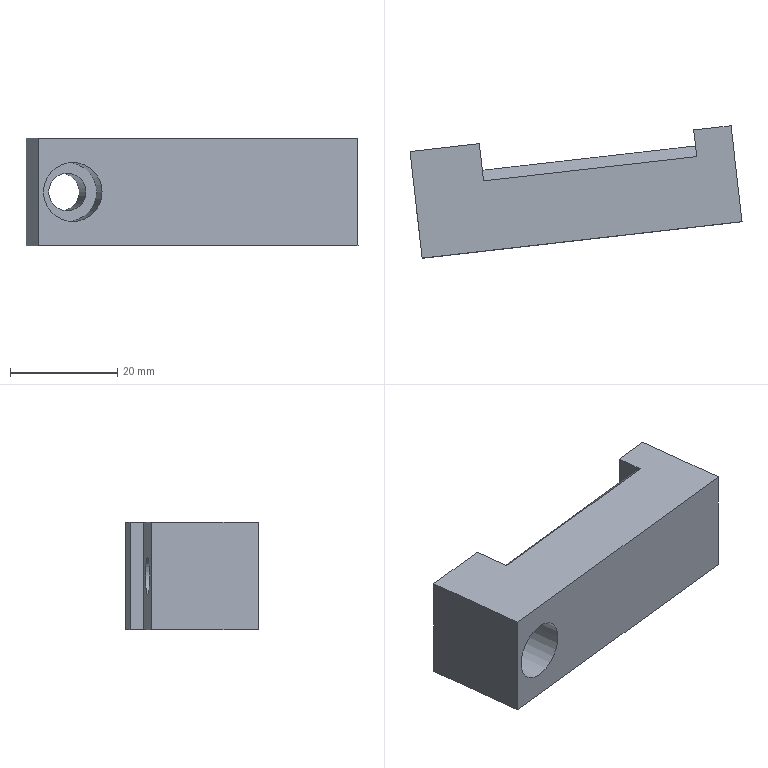Part | NX | features XQ 2 | 1 solid | 15 faces | box 61.878 x 24.676 x 20 mm | volume 18281 mm3 | plane 13 | cylinder 2 | commonest cylinder face diameters 7 x1 11 x1
STEP:
#1=CARTESIAN_POINT('',(3280.526,214.819,-94.126));
#2=VERTEX_POINT('',#1);
#3=CARTESIAN_POINT('',(3220.911,208.026,-94.126));
#4=VERTEX_POINT('',#3);
#5=CARTESIAN_POINT('',(3240.783,210.291,-94.126));
#6=DIRECTION('',(-0.9936,-0.1132,0.));
#7=VECTOR('',#6,1000.);
#8=LINE('',#5,#7);
#9=EDGE_CURVE('',#2,#4,#8,.T.);
#10=ORIENTED_EDGE('',*,*,#9,.F.);
#11=CARTESIAN_POINT('',(3280.526,214.819,-74.126));
#12=VERTEX_POINT('',#11);
#13=CARTESIAN_POINT('',(3280.526,214.819,-148.027));
#14=DIRECTION('',(0.,0.,-1.));
#15=VECTOR('',#14,1000.);
#16=LINE('',#13,#15);
#17=EDGE_CURVE('',#12,#2,#16,.T.);
#18=ORIENTED_EDGE('',*,*,#17,.F.);
#19=CARTESIAN_POINT('',(3220.911,208.026,-74.126));
#20=VERTEX_POINT('',#19);
#21=CARTESIAN_POINT('',(3240.783,210.291,-74.126));
#22=DIRECTION('',(0.9936,0.1132,0.));
#23=VECTOR('',#22,1000.);
#24=LINE('',#21,#23);
#25=EDGE_CURVE('',#20,#12,#24,.T.);
#26=ORIENTED_EDGE('',*,*,#25,.F.);
#27=CARTESIAN_POINT('',(3220.911,208.026,-94.126));
#28=DIRECTION('',(0.,0.,-1.));
#29=VECTOR('',#28,1000.);
#30=LINE('',#27,#29);
#31=EDGE_CURVE('',#20,#4,#30,.T.);
#32=ORIENTED_EDGE('',*,*,#31,.T.);
#33=EDGE_LOOP('',(#10,#18,#26,#32));
#34=FACE_BOUND('',#33,.T.);
#35=CARTESIAN_POINT('',(3232.834,209.385,-84.126));
#36=VERTEX_POINT('',#35);
#37=CARTESIAN_POINT('',(3227.369,208.762,-84.126));
#38=DIRECTION('',(0.1132,-0.9936,0.));
#39=DIRECTION('',(0.9936,0.1132,0.));
#40=AXIS2_PLACEMENT_3D('',#37,#38,#39);
#41=CIRCLE('',#40,5.5);
#42=EDGE_CURVE('',#36,#36,#41,.T.);
#43=ORIENTED_EDGE('',*,*,#42,.F.);
#44=EDGE_LOOP('',(#43));
#45=FACE_BOUND('',#44,.T.);
#46=CARTESIAN_POINT('',(3240.783,210.291,-94.126));
#47=DIRECTION('',(0.1132,-0.9936,0.));
#48=DIRECTION('',(0.9936,0.1132,0.));
#49=AXIS2_PLACEMENT_3D('',#46,#47,#48);
#50=PLANE('',#49);
#51=ADVANCED_FACE('',(#34,#45),#50,.T.);
#52=CARTESIAN_POINT('',(3231.564,229.37,-74.126));
#53=VERTEX_POINT('',#52);
#54=CARTESIAN_POINT('',(3218.647,227.898,-74.126));
#55=VERTEX_POINT('',#54);
#56=CARTESIAN_POINT('',(3236.531,229.936,-74.126));
#57=DIRECTION('',(-0.9936,-0.1132,0.));
#58=VECTOR('',#57,1000.);
#59=LINE('',#56,#58);
#60=EDGE_CURVE('',#53,#55,#59,.T.);
#61=ORIENTED_EDGE('',*,*,#60,.F.);
#62=CARTESIAN_POINT('',(3231.564,229.37,-94.126));
#63=VERTEX_POINT('',#62);
#64=CARTESIAN_POINT('',(3231.564,229.37,-94.126));
#65=DIRECTION('',(0.,0.,1.));
#66=VECTOR('',#65,1000.);
#67=LINE('',#64,#66);
#68=EDGE_CURVE('',#63,#53,#67,.T.);
#69=ORIENTED_EDGE('',*,*,#68,.F.);
#70=CARTESIAN_POINT('',(3218.647,227.898,-94.126));
#71=VERTEX_POINT('',#70);
#72=CARTESIAN_POINT('',(3236.531,229.936,-94.126));
#73=DIRECTION('',(0.9936,0.1132,0.));
#74=VECTOR('',#73,1000.);
#75=LINE('',#72,#74);
#76=EDGE_CURVE('',#71,#63,#75,.T.);
#77=ORIENTED_EDGE('',*,*,#76,.F.);
#78=CARTESIAN_POINT('',(3218.647,227.898,-94.126));
#79=DIRECTION('',(0.,0.,-1.));
#80=VECTOR('',#79,1000.);
#81=LINE('',#78,#80);
#82=EDGE_CURVE('',#55,#71,#81,.T.);
#83=ORIENTED_EDGE('',*,*,#82,.F.);
#84=EDGE_LOOP('',(#61,#69,#77,#83));
#85=FACE_BOUND('',#84,.T.);
#86=CARTESIAN_POINT('',(3221.628,228.237,-84.126));
#87=VERTEX_POINT('',#86);
#88=CARTESIAN_POINT('',(3225.105,228.634,-84.126));
#89=DIRECTION('',(-0.1132,0.9936,0.));
#90=DIRECTION('',(-0.9936,-0.1132,0.));
#91=AXIS2_PLACEMENT_3D('',#88,#89,#90);
#92=CIRCLE('',#91,3.5);
#93=EDGE_CURVE('',#87,#87,#92,.T.);
#94=ORIENTED_EDGE('',*,*,#93,.F.);
#95=EDGE_LOOP('',(#94));
#96=FACE_BOUND('',#95,.T.);
#97=CARTESIAN_POINT('',(3236.531,229.936,-94.126));
#98=DIRECTION('',(-0.1132,0.9936,0.));
#99=DIRECTION('',(-0.9936,-0.1132,0.));
#100=AXIS2_PLACEMENT_3D('',#97,#98,#99);
#101=PLANE('',#100);
#102=ADVANCED_FACE('',(#85,#96),#101,.T.);
#103=CARTESIAN_POINT('',(3272.099,226.943,-74.126));
#104=VERTEX_POINT('',#103);
#105=CARTESIAN_POINT('',(3232.356,222.415,-74.126));
#106=VERTEX_POINT('',#105);
#107=CARTESIAN_POINT('',(3239.311,223.207,-74.126));
#108=DIRECTION('',(-0.9936,-0.1132,0.));
#109=VECTOR('',#108,1000.);
#110=LINE('',#107,#109);
#111=EDGE_CURVE('',#104,#106,#110,.T.);
#112=ORIENTED_EDGE('',*,*,#111,.T.);
#113=CARTESIAN_POINT('',(3232.696,219.434,-74.126));
#114=DIRECTION('',(-0.1132,0.9936,0.));
#115=VECTOR('',#114,1000.);
#116=LINE('',#113,#115);
#117=EDGE_CURVE('',#106,#53,#116,.T.);
#118=ORIENTED_EDGE('',*,*,#117,.T.);
#119=ORIENTED_EDGE('',*,*,#60,.T.);
#120=CARTESIAN_POINT('',(3219.779,217.962,-74.126));
#121=DIRECTION('',(0.1132,-0.9936,0.));
#122=VECTOR('',#121,1000.);
#123=LINE('',#120,#122);
#124=EDGE_CURVE('',#55,#20,#123,.T.);
#125=ORIENTED_EDGE('',*,*,#124,.T.);
#126=ORIENTED_EDGE('',*,*,#25,.T.);
#127=CARTESIAN_POINT('',(3278.488,232.703,-74.126));
#128=VERTEX_POINT('',#127);
#129=CARTESIAN_POINT('',(3279.394,224.754,-74.126));
#130=DIRECTION('',(-0.1132,0.9936,0.));
#131=VECTOR('',#130,1000.);
#132=LINE('',#129,#131);
#133=EDGE_CURVE('',#12,#128,#132,.T.);
#134=ORIENTED_EDGE('',*,*,#133,.T.);
#135=CARTESIAN_POINT('',(3271.533,231.91,-74.126));
#136=VERTEX_POINT('',#135);
#137=CARTESIAN_POINT('',(3238.745,228.175,-74.126));
#138=DIRECTION('',(-0.9936,-0.1132,0.));
#139=VECTOR('',#138,1000.);
#140=LINE('',#137,#139);
#141=EDGE_CURVE('',#128,#136,#140,.T.);
#142=ORIENTED_EDGE('',*,*,#141,.T.);
#143=CARTESIAN_POINT('',(3272.439,223.962,-74.126));
#144=DIRECTION('',(0.1132,-0.9936,0.));
#145=VECTOR('',#144,1000.);
#146=LINE('',#143,#145);
#147=EDGE_CURVE('',#136,#104,#146,.T.);
#148=ORIENTED_EDGE('',*,*,#147,.T.);
#149=EDGE_LOOP('',(#112,#118,#119,#125,#126,#134,#142,#148));
#150=FACE_BOUND('',#149,.T.);
#151=CARTESIAN_POINT('',(3239.651,220.226,-74.126));
#152=DIRECTION('',(0.,0.,1.));
#153=DIRECTION('',(-0.9981,0.06105,0.));
#154=AXIS2_PLACEMENT_3D('',#151,#152,#153);
#155=PLANE('',#154);
#156=ADVANCED_FACE('',(#150),#155,.T.);
#157=CARTESIAN_POINT('',(3271.873,228.93,-76.126));
#158=VERTEX_POINT('',#157);
#159=CARTESIAN_POINT('',(3271.873,228.93,-92.126));
#160=VERTEX_POINT('',#159);
#161=CARTESIAN_POINT('',(3271.873,228.93,-84.126));
#162=DIRECTION('',(0.,0.,-1.));
#163=VECTOR('',#162,1000.);
#164=LINE('',#161,#163);
#165=EDGE_CURVE('',#158,#160,#164,.T.);
#166=ORIENTED_EDGE('',*,*,#165,.T.);
#167=CARTESIAN_POINT('',(3232.13,224.402,-92.126));
#168=VERTEX_POINT('',#167);
#169=CARTESIAN_POINT('',(3239.085,225.194,-92.126));
#170=DIRECTION('',(-0.9936,-0.1132,0.));
#171=VECTOR('',#170,1000.);
#172=LINE('',#169,#171);
#173=EDGE_CURVE('',#160,#168,#172,.T.);
#174=ORIENTED_EDGE('',*,*,#173,.T.);
#175=CARTESIAN_POINT('',(3232.13,224.402,-76.126));
#176=VERTEX_POINT('',#175);
#177=CARTESIAN_POINT('',(3232.13,224.402,-84.126));
#178=DIRECTION('',(0.,0.,-1.));
#179=VECTOR('',#178,1000.);
#180=LINE('',#177,#179);
#181=EDGE_CURVE('',#176,#168,#180,.T.);
#182=ORIENTED_EDGE('',*,*,#181,.F.);
#183=CARTESIAN_POINT('',(3239.085,225.194,-76.126));
#184=DIRECTION('',(0.9936,0.1132,0.));
#185=VECTOR('',#184,1000.);
#186=LINE('',#183,#185);
#187=EDGE_CURVE('',#176,#158,#186,.T.);
#188=ORIENTED_EDGE('',*,*,#187,.T.);
#189=EDGE_LOOP('',(#166,#174,#182,#188));
#190=FACE_BOUND('',#189,.T.);
#191=CARTESIAN_POINT('',(3239.085,225.194,-94.126));
#192=DIRECTION('',(-0.1132,0.9936,0.));
#193=DIRECTION('',(-0.9936,-0.1132,0.));
#194=AXIS2_PLACEMENT_3D('',#191,#192,#193);
#195=PLANE('',#194);
#196=ADVANCED_FACE('',(#190),#195,.T.);
#197=CARTESIAN_POINT('',(3232.356,222.415,-94.126));
#198=VERTEX_POINT('',#197);
#199=CARTESIAN_POINT('',(3272.099,226.943,-94.126));
#200=VERTEX_POINT('',#199);
#201=CARTESIAN_POINT('',(3239.311,223.207,-94.126));
#202=DIRECTION('',(0.9936,0.1132,0.));
#203=VECTOR('',#202,1000.);
#204=LINE('',#201,#203);
#205=EDGE_CURVE('',#198,#200,#204,.T.);
#206=ORIENTED_EDGE('',*,*,#205,.T.);
#207=CARTESIAN_POINT('',(3271.533,231.91,-94.126));
#208=VERTEX_POINT('',#207);
#209=CARTESIAN_POINT('',(3272.439,223.962,-94.126));
#210=DIRECTION('',(0.1132,-0.9936,0.));
#211=VECTOR('',#210,1000.);
#212=LINE('',#209,#211);
#213=EDGE_CURVE('',#208,#200,#212,.T.);
#214=ORIENTED_EDGE('',*,*,#213,.F.);
#215=CARTESIAN_POINT('',(3278.488,232.703,-94.126));
#216=VERTEX_POINT('',#215);
#217=CARTESIAN_POINT('',(3238.745,228.175,-94.126));
#218=DIRECTION('',(0.9936,0.1132,0.));
#219=VECTOR('',#218,1000.);
#220=LINE('',#217,#219);
#221=EDGE_CURVE('',#208,#216,#220,.T.);
#222=ORIENTED_EDGE('',*,*,#221,.T.);
#223=CARTESIAN_POINT('',(3279.394,224.754,-94.126));
#224=DIRECTION('',(0.1132,-0.9936,0.));
#225=VECTOR('',#224,1000.);
#226=LINE('',#223,#225);
#227=EDGE_CURVE('',#216,#2,#226,.T.);
#228=ORIENTED_EDGE('',*,*,#227,.T.);
#229=ORIENTED_EDGE('',*,*,#9,.T.);
#230=CARTESIAN_POINT('',(3219.779,217.962,-94.126));
#231=DIRECTION('',(-0.1132,0.9936,0.));
#232=VECTOR('',#231,1000.);
#233=LINE('',#230,#232);
#234=EDGE_CURVE('',#4,#71,#233,.T.);
#235=ORIENTED_EDGE('',*,*,#234,.T.);
#236=ORIENTED_EDGE('',*,*,#76,.T.);
#237=CARTESIAN_POINT('',(3232.696,219.434,-94.126));
#238=DIRECTION('',(0.1132,-0.9936,0.));
#239=VECTOR('',#238,1000.);
#240=LINE('',#237,#239);
#241=EDGE_CURVE('',#63,#198,#240,.T.);
#242=ORIENTED_EDGE('',*,*,#241,.T.);
#243=EDGE_LOOP('',(#206,#214,#222,#228,#229,#235,#236,#242));
#244=FACE_BOUND('',#243,.T.);
#245=CARTESIAN_POINT('',(3239.651,220.226,-94.126));
#246=DIRECTION('',(0.,0.,-1.));
#247=DIRECTION('',(0.9981,-0.06105,0.));
#248=AXIS2_PLACEMENT_3D('',#245,#246,#247);
#249=PLANE('',#248);
#250=ADVANCED_FACE('',(#244),#249,.T.);
#251=ORIENTED_EDGE('',*,*,#241,.F.);
#252=ORIENTED_EDGE('',*,*,#68,.T.);
#253=ORIENTED_EDGE('',*,*,#117,.F.);
#254=CARTESIAN_POINT('',(3232.356,222.415,-74.126));
#255=DIRECTION('',(-0.08005,0.7026,-0.7071));
#256=VECTOR('',#255,1000.);
#257=LINE('',#254,#256);
#258=EDGE_CURVE('',#106,#176,#257,.T.);
#259=ORIENTED_EDGE('',*,*,#258,.T.);
#260=ORIENTED_EDGE('',*,*,#181,.T.);
#261=CARTESIAN_POINT('',(3232.356,222.415,-94.126));
#262=DIRECTION('',(0.08005,-0.7026,-0.7071));
#263=VECTOR('',#262,1000.);
#264=LINE('',#261,#263);
#265=EDGE_CURVE('',#168,#198,#264,.T.);
#266=ORIENTED_EDGE('',*,*,#265,.T.);
#267=EDGE_LOOP('',(#251,#252,#253,#259,#260,#266));
#268=FACE_BOUND('',#267,.T.);
#269=CARTESIAN_POINT('',(3232.413,221.918,-84.126));
#270=DIRECTION('',(0.9936,0.1132,0.));
#271=DIRECTION('',(-0.1132,0.9936,0.));
#272=AXIS2_PLACEMENT_3D('',#269,#270,#271);
#273=PLANE('',#272);
#274=ADVANCED_FACE('',(#268),#273,.T.);
#275=ORIENTED_EDGE('',*,*,#31,.F.);
#276=ORIENTED_EDGE('',*,*,#124,.F.);
#277=ORIENTED_EDGE('',*,*,#82,.T.);
#278=ORIENTED_EDGE('',*,*,#234,.F.);
#279=EDGE_LOOP('',(#275,#276,#277,#278));
#280=FACE_BOUND('',#279,.T.);
#281=CARTESIAN_POINT('',(3219.779,217.962,-94.126));
#282=DIRECTION('',(-0.9936,-0.1132,0.));
#283=DIRECTION('',(0.1132,-0.9936,0.));
#284=AXIS2_PLACEMENT_3D('',#281,#282,#283);
#285=PLANE('',#284);
#286=ADVANCED_FACE('',(#280),#285,.T.);
#287=ORIENTED_EDGE('',*,*,#213,.T.);
#288=CARTESIAN_POINT('',(3272.099,226.943,-94.126));
#289=DIRECTION('',(-0.08005,0.7026,0.7071));
#290=VECTOR('',#289,1000.);
#291=LINE('',#288,#290);
#292=EDGE_CURVE('',#200,#160,#291,.T.);
#293=ORIENTED_EDGE('',*,*,#292,.T.);
#294=ORIENTED_EDGE('',*,*,#165,.F.);
#295=CARTESIAN_POINT('',(3272.099,226.943,-74.126));
#296=DIRECTION('',(0.08005,-0.7026,0.7071));
#297=VECTOR('',#296,1000.);
#298=LINE('',#295,#297);
#299=EDGE_CURVE('',#158,#104,#298,.T.);
#300=ORIENTED_EDGE('',*,*,#299,.T.);
#301=ORIENTED_EDGE('',*,*,#147,.F.);
#302=CARTESIAN_POINT('',(3271.533,231.91,-94.126));
#303=DIRECTION('',(0.,0.,1.));
#304=VECTOR('',#303,1000.);
#305=LINE('',#302,#304);
#306=EDGE_CURVE('',#208,#136,#305,.T.);
#307=ORIENTED_EDGE('',*,*,#306,.F.);
#308=EDGE_LOOP('',(#287,#293,#294,#300,#301,#307));
#309=FACE_BOUND('',#308,.T.);
#310=CARTESIAN_POINT('',(3272.439,223.962,-84.126));
#311=DIRECTION('',(-0.9936,-0.1132,0.));
#312=DIRECTION('',(0.1132,-0.9936,0.));
#313=AXIS2_PLACEMENT_3D('',#310,#311,#312);
#314=PLANE('',#313);
#315=ADVANCED_FACE('',(#309),#314,.T.);
#316=ORIENTED_EDGE('',*,*,#227,.F.);
#317=CARTESIAN_POINT('',(3278.488,232.703,-94.126));
#318=DIRECTION('',(0.,0.,-1.));
#319=VECTOR('',#318,1000.);
#320=LINE('',#317,#319);
#321=EDGE_CURVE('',#128,#216,#320,.T.);
#322=ORIENTED_EDGE('',*,*,#321,.F.);
#323=ORIENTED_EDGE('',*,*,#133,.F.);
#324=ORIENTED_EDGE('',*,*,#17,.T.);
#325=EDGE_LOOP('',(#316,#322,#323,#324));
#326=FACE_BOUND('',#325,.T.);
#327=CARTESIAN_POINT('',(3255.338,435.888,-148.027));
#328=DIRECTION('',(0.9936,0.1132,0.));
#329=DIRECTION('',(0.,0.,1.));
#330=AXIS2_PLACEMENT_3D('',#327,#328,#329);
#331=PLANE('',#330);
#332=ADVANCED_FACE('',(#326),#331,.T.);
#333=ORIENTED_EDGE('',*,*,#221,.F.);
#334=ORIENTED_EDGE('',*,*,#306,.T.);
#335=ORIENTED_EDGE('',*,*,#141,.F.);
#336=ORIENTED_EDGE('',*,*,#321,.T.);
#337=EDGE_LOOP('',(#333,#334,#335,#336));
#338=FACE_BOUND('',#337,.T.);
#339=CARTESIAN_POINT('',(3238.745,228.175,-94.126));
#340=DIRECTION('',(-0.1132,0.9936,0.));
#341=DIRECTION('',(-0.9936,-0.1132,0.));
#342=AXIS2_PLACEMENT_3D('',#339,#340,#341);
#343=PLANE('',#342);
#344=ADVANCED_FACE('',(#338),#343,.T.);
#345=CARTESIAN_POINT('',(3222.873,217.308,-84.126));
#346=VERTEX_POINT('',#345);
#347=CARTESIAN_POINT('',(3226.351,217.704,-84.126));
#348=DIRECTION('',(0.1132,-0.9936,0.));
#349=DIRECTION('',(-0.9936,-0.1132,0.));
#350=AXIS2_PLACEMENT_3D('',#347,#348,#349);
#351=CIRCLE('',#350,3.5);
#352=EDGE_CURVE('',#346,#346,#351,.T.);
#353=ORIENTED_EDGE('',*,*,#352,.T.);
#354=EDGE_LOOP('',(#353));
#355=FACE_BOUND('',#354,.T.);
#356=ORIENTED_EDGE('',*,*,#93,.T.);
#357=EDGE_LOOP('',(#356));
#358=FACE_BOUND('',#357,.T.);
#359=CARTESIAN_POINT('',(3227.369,208.762,-84.126));
#360=DIRECTION('',(-0.1132,0.9936,0.));
#361=DIRECTION('',(-0.9785,-0.1115,-0.1736));
#362=AXIS2_PLACEMENT_3D('',#359,#360,#361);
#363=CYLINDRICAL_SURFACE('',#362,3.5);
#364=ADVANCED_FACE('',(#355,#358),#363,.F.);
#365=ORIENTED_EDGE('',*,*,#352,.F.);
#366=EDGE_LOOP('',(#365));
#367=FACE_BOUND('',#366,.T.);
#368=CARTESIAN_POINT('',(3220.886,217.082,-84.126));
#369=VERTEX_POINT('',#368);
#370=CARTESIAN_POINT('',(3226.351,217.704,-84.126));
#371=DIRECTION('',(0.1132,-0.9936,0.));
#372=DIRECTION('',(-0.9936,-0.1132,0.));
#373=AXIS2_PLACEMENT_3D('',#370,#371,#372);
#374=CIRCLE('',#373,5.5);
#375=EDGE_CURVE('',#369,#369,#374,.T.);
#376=ORIENTED_EDGE('',*,*,#375,.T.);
#377=EDGE_LOOP('',(#376));
#378=FACE_BOUND('',#377,.T.);
#379=CARTESIAN_POINT('',(3226.351,217.704,-84.126));
#380=DIRECTION('',(-0.1132,0.9936,0.));
#381=DIRECTION('',(-0.9936,-0.1132,0.));
#382=AXIS2_PLACEMENT_3D('',#379,#380,#381);
#383=PLANE('',#382);
#384=ADVANCED_FACE('',(#367,#378),#383,.F.);
#385=ORIENTED_EDGE('',*,*,#375,.F.);
#386=EDGE_LOOP('',(#385));
#387=FACE_BOUND('',#386,.T.);
#388=ORIENTED_EDGE('',*,*,#42,.T.);
#389=EDGE_LOOP('',(#388));
#390=FACE_BOUND('',#389,.T.);
#391=CARTESIAN_POINT('',(3227.369,208.762,-84.126));
#392=DIRECTION('',(-0.1132,0.9936,0.));
#393=DIRECTION('',(-0.9785,-0.1115,-0.1736));
#394=AXIS2_PLACEMENT_3D('',#391,#392,#393);
#395=CYLINDRICAL_SURFACE('',#394,5.5);
#396=ADVANCED_FACE('',(#387,#390),#395,.F.);
#397=ORIENTED_EDGE('',*,*,#258,.F.);
#398=ORIENTED_EDGE('',*,*,#111,.F.);
#399=ORIENTED_EDGE('',*,*,#299,.F.);
#400=ORIENTED_EDGE('',*,*,#187,.F.);
#401=EDGE_LOOP('',(#397,#398,#399,#400));
#402=FACE_BOUND('',#401,.T.);
#403=CARTESIAN_POINT('',(3239.311,223.207,-74.126));
#404=DIRECTION('',(0.08005,-0.7026,-0.7071));
#405=DIRECTION('',(0.9936,0.1132,0.));
#406=AXIS2_PLACEMENT_3D('',#403,#404,#405);
#407=PLANE('',#406);
#408=ADVANCED_FACE('',(#402),#407,.F.);
#409=ORIENTED_EDGE('',*,*,#292,.F.);
#410=ORIENTED_EDGE('',*,*,#205,.F.);
#411=ORIENTED_EDGE('',*,*,#265,.F.);
#412=ORIENTED_EDGE('',*,*,#173,.F.);
#413=EDGE_LOOP('',(#409,#410,#411,#412));
#414=FACE_BOUND('',#413,.T.);
#415=CARTESIAN_POINT('',(3239.311,223.207,-94.126));
#416=DIRECTION('',(0.08005,-0.7026,0.7071));
#417=DIRECTION('',(-0.9936,-0.1132,0.));
#418=AXIS2_PLACEMENT_3D('',#415,#416,#417);
#419=PLANE('',#418);
#420=ADVANCED_FACE('',(#414),#419,.F.);
#421=CLOSED_SHELL('',(#51,#102,#156,#196,#250,#274,#286,#315,#332,#344,#364,#384,#396,#408,#420));
#422=MANIFOLD_SOLID_BREP('',#421);
#423=(LENGTH_UNIT()NAMED_UNIT(*)SI_UNIT(.MILLI.,.METRE.));
#424=UNCERTAINTY_MEASURE_WITH_UNIT(LENGTH_MEASURE(0.00001),#423,'','');
#425=(NAMED_UNIT(*)PLANE_ANGLE_UNIT()SI_UNIT($,.RADIAN.));
#426=(NAMED_UNIT(*)SI_UNIT($,.STERADIAN.)SOLID_ANGLE_UNIT());
#427=(GEOMETRIC_REPRESENTATION_CONTEXT(3)GLOBAL_UNCERTAINTY_ASSIGNED_CONTEXT((#424))GLOBAL_UNIT_ASSIGNED_CONTEXT((#423,#425,#426))REPRESENTATION_CONTEXT('',''));
#428=ADVANCED_BREP_SHAPE_REPRESENTATION('',(#422),#427);